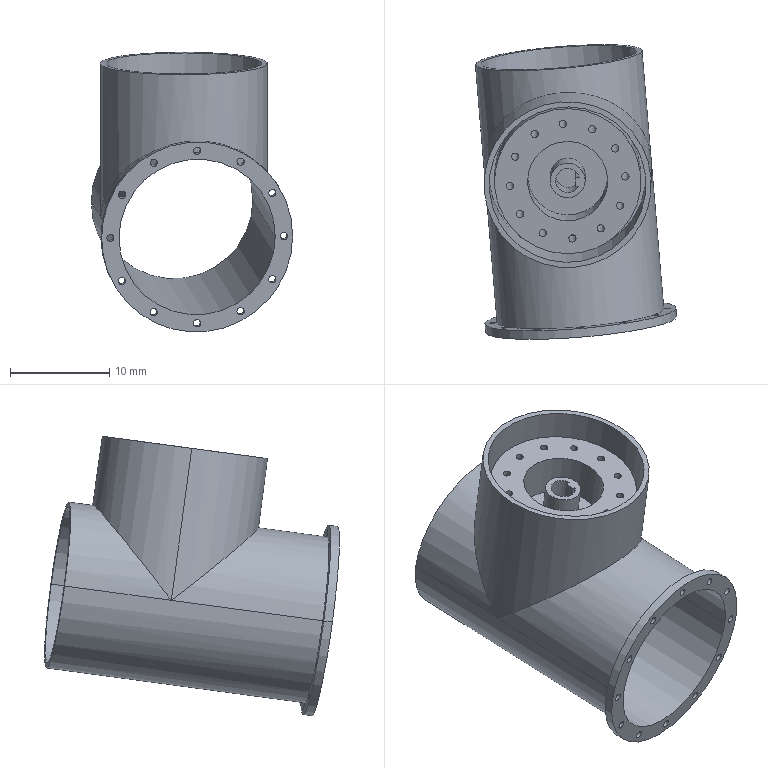Part | SolidWorks | features SplitBody 1 | 1 solid | 94 faces | box 20.334 x 29.788 x 28.252 mm | volume 1793 mm3 | cylinder 68 | plane 26 | commonest cylinder face diameters 0.739 x48 16.896 x5 15.84 x4 3.52 x3 2.464 x2 8.096 x2